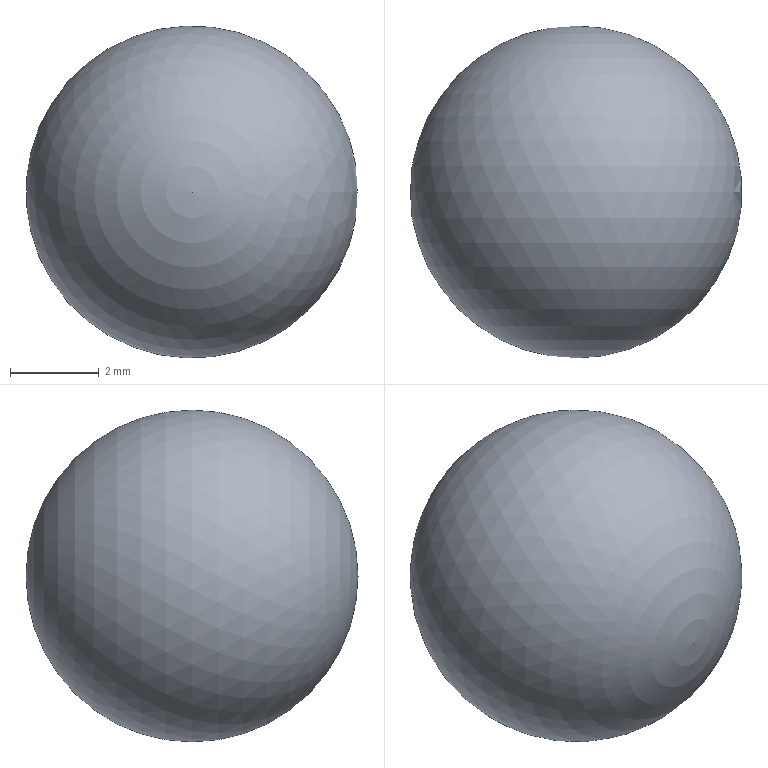Part | STEP file | Ball | 1 solid | 1 faces | box 7.5 x 7.5 x 7.5 mm | volume 220.893 mm3 | sphere 1
STEP:
#1=CARTESIAN_POINT('',(0.,33.75,0.));
#2=DIRECTION('',(0.,-1.,0.));
#3=DIRECTION('',(1.,0.,0.));
#4=AXIS2_PLACEMENT_3D('',#1,#2,#3);
#5=SPHERICAL_SURFACE('',#4,3.75);
#6=ADVANCED_FACE('',(),#5,.T.);
#7=CLOSED_SHELL('',(#6));
#8=MANIFOLD_SOLID_BREP('',#7);
#9=(LENGTH_UNIT()NAMED_UNIT(*)SI_UNIT(.MILLI.,.METRE.));
#10=UNCERTAINTY_MEASURE_WITH_UNIT(LENGTH_MEASURE(0.00001),#9,'','');
#11=(NAMED_UNIT(*)PLANE_ANGLE_UNIT()SI_UNIT($,.RADIAN.));
#12=(NAMED_UNIT(*)SI_UNIT($,.STERADIAN.)SOLID_ANGLE_UNIT());
#13=(GEOMETRIC_REPRESENTATION_CONTEXT(3)GLOBAL_UNCERTAINTY_ASSIGNED_CONTEXT((#10))GLOBAL_UNIT_ASSIGNED_CONTEXT((#9,#11,#12))REPRESENTATION_CONTEXT('',''));
#14=ADVANCED_BREP_SHAPE_REPRESENTATION('',(#8),#13);